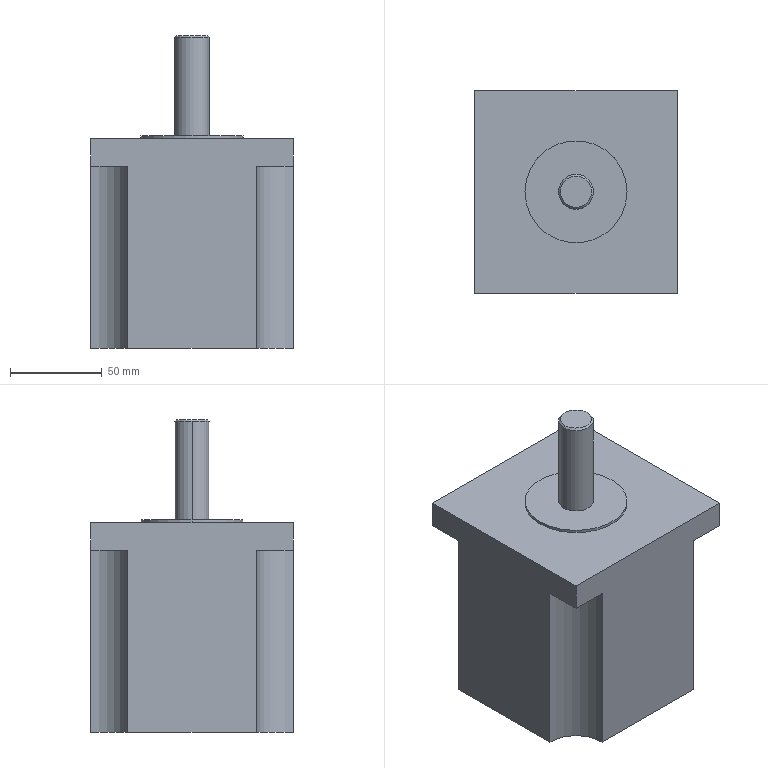Part | STEP file | Guide wheel mechanism revised.sldasm-Part-355 | 1 solid | 22 faces | box 110 x 110 x 170 mm | volume 1274045 mm3 | plane 12 | cylinder 8 | cone 2 | commonest cylinder face diameters 40 x4 19 x2 55.5 x2
STEP:
#1=CARTESIAN_POINT('',(8.5,0.,56.));
#2=VERTEX_POINT('',#1);
#3=CARTESIAN_POINT('',(-8.5,0.,56.));
#4=VERTEX_POINT('',#3);
#5=CARTESIAN_POINT('',(0.,0.,56.));
#6=DIRECTION('',(0.,0.,1.));
#7=DIRECTION('',(1.,0.,0.));
#8=AXIS2_PLACEMENT_3D('',#5,#6,#7);
#9=CIRCLE('',#8,8.5);
#10=EDGE_CURVE('',#2,#4,#9,.T.);
#11=ORIENTED_EDGE('',*,*,#10,.F.);
#12=CARTESIAN_POINT('',(9.5,0.,55.));
#13=VERTEX_POINT('',#12);
#14=CARTESIAN_POINT('',(8.5,0.,56.));
#15=DIRECTION('',(0.7071,0.,-0.7071));
#16=VECTOR('',#15,1000.);
#17=LINE('',#14,#16);
#18=EDGE_CURVE('',#2,#13,#17,.T.);
#19=ORIENTED_EDGE('',*,*,#18,.T.);
#20=CARTESIAN_POINT('',(-9.5,0.,55.));
#21=VERTEX_POINT('',#20);
#22=CARTESIAN_POINT('',(0.,0.,55.));
#23=DIRECTION('',(0.,0.,-1.));
#24=DIRECTION('',(1.,0.,0.));
#25=AXIS2_PLACEMENT_3D('',#22,#23,#24);
#26=CIRCLE('',#25,9.5);
#27=EDGE_CURVE('',#21,#13,#26,.T.);
#28=ORIENTED_EDGE('',*,*,#27,.F.);
#29=CARTESIAN_POINT('',(-8.5,0.,56.));
#30=DIRECTION('',(-0.7071,0.,-0.7071));
#31=VECTOR('',#30,1000.);
#32=LINE('',#29,#31);
#33=EDGE_CURVE('',#4,#21,#32,.T.);
#34=ORIENTED_EDGE('',*,*,#33,.F.);
#35=EDGE_LOOP('',(#11,#19,#28,#34));
#36=FACE_OUTER_BOUND('',#35,.T.);
#37=CARTESIAN_POINT('',(0.,0.,56.));
#38=DIRECTION('',(0.,0.,-1.));
#39=DIRECTION('',(-1.,0.,0.));
#40=AXIS2_PLACEMENT_3D('',#37,#38,#39);
#41=CONICAL_SURFACE('',#40,8.5,0.7854);
#42=ADVANCED_FACE('',(#36),#41,.T.);
#43=ORIENTED_EDGE('',*,*,#27,.T.);
#44=CARTESIAN_POINT('',(9.5,0.,1.5));
#45=VERTEX_POINT('',#44);
#46=CARTESIAN_POINT('',(9.5,0.,56.));
#47=DIRECTION('',(0.,0.,-1.));
#48=VECTOR('',#47,1000.);
#49=LINE('',#46,#48);
#50=EDGE_CURVE('',#13,#45,#49,.T.);
#51=ORIENTED_EDGE('',*,*,#50,.T.);
#52=CARTESIAN_POINT('',(-9.5,0.,1.5));
#53=VERTEX_POINT('',#52);
#54=CARTESIAN_POINT('',(0.,0.,1.5));
#55=DIRECTION('',(0.,0.,1.));
#56=DIRECTION('',(1.,0.,0.));
#57=AXIS2_PLACEMENT_3D('',#54,#55,#56);
#58=CIRCLE('',#57,9.5);
#59=EDGE_CURVE('',#45,#53,#58,.T.);
#60=ORIENTED_EDGE('',*,*,#59,.T.);
#61=CARTESIAN_POINT('',(-9.5,0.,56.));
#62=DIRECTION('',(0.,0.,-1.));
#63=VECTOR('',#62,1000.);
#64=LINE('',#61,#63);
#65=EDGE_CURVE('',#21,#53,#64,.T.);
#66=ORIENTED_EDGE('',*,*,#65,.F.);
#67=EDGE_LOOP('',(#43,#51,#60,#66));
#68=FACE_OUTER_BOUND('',#67,.T.);
#69=CARTESIAN_POINT('',(0.,0.,56.));
#70=DIRECTION('',(0.,0.,-1.));
#71=DIRECTION('',(-1.,0.,0.));
#72=AXIS2_PLACEMENT_3D('',#69,#70,#71);
#73=CYLINDRICAL_SURFACE('',#72,9.5);
#74=ADVANCED_FACE('',(#68),#73,.T.);
#75=CARTESIAN_POINT('',(27.75,0.,1.5));
#76=VERTEX_POINT('',#75);
#77=CARTESIAN_POINT('',(-27.75,0.,1.5));
#78=VERTEX_POINT('',#77);
#79=CARTESIAN_POINT('',(0.,0.,1.5));
#80=DIRECTION('',(0.,0.,1.));
#81=DIRECTION('',(1.,0.,0.));
#82=AXIS2_PLACEMENT_3D('',#79,#80,#81);
#83=CIRCLE('',#82,27.75);
#84=EDGE_CURVE('',#76,#78,#83,.T.);
#85=ORIENTED_EDGE('',*,*,#84,.F.);
#86=CARTESIAN_POINT('',(27.75,0.,0.));
#87=VERTEX_POINT('',#86);
#88=CARTESIAN_POINT('',(27.75,0.,1.5));
#89=DIRECTION('',(0.,0.,-1.));
#90=VECTOR('',#89,1000.);
#91=LINE('',#88,#90);
#92=EDGE_CURVE('',#76,#87,#91,.T.);
#93=ORIENTED_EDGE('',*,*,#92,.T.);
#94=CARTESIAN_POINT('',(-27.75,0.,0.));
#95=VERTEX_POINT('',#94);
#96=CARTESIAN_POINT('',(0.,0.,0.));
#97=DIRECTION('',(0.,0.,1.));
#98=DIRECTION('',(1.,0.,0.));
#99=AXIS2_PLACEMENT_3D('',#96,#97,#98);
#100=CIRCLE('',#99,27.75);
#101=EDGE_CURVE('',#87,#95,#100,.T.);
#102=ORIENTED_EDGE('',*,*,#101,.T.);
#103=CARTESIAN_POINT('',(-27.75,0.,1.5));
#104=DIRECTION('',(0.,0.,-1.));
#105=VECTOR('',#104,1000.);
#106=LINE('',#103,#105);
#107=EDGE_CURVE('',#78,#95,#106,.T.);
#108=ORIENTED_EDGE('',*,*,#107,.F.);
#109=EDGE_LOOP('',(#85,#93,#102,#108));
#110=FACE_OUTER_BOUND('',#109,.T.);
#111=CARTESIAN_POINT('',(0.,0.,1.5));
#112=DIRECTION('',(0.,0.,-1.));
#113=DIRECTION('',(-1.,0.,0.));
#114=AXIS2_PLACEMENT_3D('',#111,#112,#113);
#115=CYLINDRICAL_SURFACE('',#114,27.75);
#116=ADVANCED_FACE('',(#110),#115,.T.);
#117=CARTESIAN_POINT('',(-55.,-55.,0.));
#118=VERTEX_POINT('',#117);
#119=CARTESIAN_POINT('',(-55.,55.,0.));
#120=VERTEX_POINT('',#119);
#121=CARTESIAN_POINT('',(-55.,0.,0.));
#122=DIRECTION('',(0.,1.,0.));
#123=VECTOR('',#122,1000.);
#124=LINE('',#121,#123);
#125=EDGE_CURVE('',#118,#120,#124,.T.);
#126=ORIENTED_EDGE('',*,*,#125,.F.);
#127=CARTESIAN_POINT('',(55.,-55.,0.));
#128=VERTEX_POINT('',#127);
#129=CARTESIAN_POINT('',(0.,-55.,0.));
#130=DIRECTION('',(-1.,0.,0.));
#131=VECTOR('',#130,1000.);
#132=LINE('',#129,#131);
#133=EDGE_CURVE('',#128,#118,#132,.T.);
#134=ORIENTED_EDGE('',*,*,#133,.F.);
#135=CARTESIAN_POINT('',(55.,55.,0.));
#136=VERTEX_POINT('',#135);
#137=CARTESIAN_POINT('',(55.,0.,0.));
#138=DIRECTION('',(0.,1.,0.));
#139=VECTOR('',#138,1000.);
#140=LINE('',#137,#139);
#141=EDGE_CURVE('',#128,#136,#140,.T.);
#142=ORIENTED_EDGE('',*,*,#141,.T.);
#143=CARTESIAN_POINT('',(0.,55.,0.));
#144=DIRECTION('',(-1.,0.,0.));
#145=VECTOR('',#144,1000.);
#146=LINE('',#143,#145);
#147=EDGE_CURVE('',#136,#120,#146,.T.);
#148=ORIENTED_EDGE('',*,*,#147,.T.);
#149=EDGE_LOOP('',(#126,#134,#142,#148));
#150=FACE_OUTER_BOUND('',#149,.T.);
#151=CARTESIAN_POINT('',(0.,0.,0.));
#152=DIRECTION('',(0.,0.,1.));
#153=DIRECTION('',(1.,0.,0.));
#154=AXIS2_PLACEMENT_3D('',#151,#152,#153);
#155=CIRCLE('',#154,27.75);
#156=EDGE_CURVE('',#95,#87,#155,.T.);
#157=ORIENTED_EDGE('',*,*,#156,.F.);
#158=ORIENTED_EDGE('',*,*,#101,.F.);
#159=EDGE_LOOP('',(#157,#158));
#160=FACE_BOUND('',#159,.T.);
#161=CARTESIAN_POINT('',(0.,0.,0.));
#162=DIRECTION('',(0.,0.,1.));
#163=DIRECTION('',(1.,0.,0.));
#164=AXIS2_PLACEMENT_3D('',#161,#162,#163);
#165=PLANE('',#164);
#166=ADVANCED_FACE('',(#150,#160),#165,.T.);
#167=CARTESIAN_POINT('',(-55.,-35.,-15.));
#168=VERTEX_POINT('',#167);
#169=CARTESIAN_POINT('',(-35.,-55.,-15.));
#170=VERTEX_POINT('',#169);
#171=CARTESIAN_POINT('',(-55.,-55.,-15.));
#172=DIRECTION('',(0.,0.,-1.));
#173=DIRECTION('',(1.,0.,0.));
#174=AXIS2_PLACEMENT_3D('',#171,#172,#173);
#175=CIRCLE('',#174,20.);
#176=EDGE_CURVE('',#168,#170,#175,.T.);
#177=ORIENTED_EDGE('',*,*,#176,.F.);
#178=CARTESIAN_POINT('',(-55.,-35.,-114.));
#179=VERTEX_POINT('',#178);
#180=CARTESIAN_POINT('',(-55.,-35.,-114.));
#181=DIRECTION('',(0.,0.,1.));
#182=VECTOR('',#181,1000.);
#183=LINE('',#180,#182);
#184=EDGE_CURVE('',#179,#168,#183,.T.);
#185=ORIENTED_EDGE('',*,*,#184,.F.);
#186=CARTESIAN_POINT('',(-35.,-55.,-114.));
#187=VERTEX_POINT('',#186);
#188=CARTESIAN_POINT('',(-55.,-55.,-114.));
#189=DIRECTION('',(0.,0.,1.));
#190=DIRECTION('',(1.,0.,0.));
#191=AXIS2_PLACEMENT_3D('',#188,#189,#190);
#192=CIRCLE('',#191,20.);
#193=EDGE_CURVE('',#187,#179,#192,.T.);
#194=ORIENTED_EDGE('',*,*,#193,.F.);
#195=CARTESIAN_POINT('',(-35.,-55.,-114.));
#196=DIRECTION('',(0.,0.,1.));
#197=VECTOR('',#196,1000.);
#198=LINE('',#195,#197);
#199=EDGE_CURVE('',#187,#170,#198,.T.);
#200=ORIENTED_EDGE('',*,*,#199,.T.);
#201=EDGE_LOOP('',(#177,#185,#194,#200));
#202=FACE_OUTER_BOUND('',#201,.T.);
#203=CARTESIAN_POINT('',(-55.,-55.,-114.));
#204=DIRECTION('',(0.,0.,1.));
#205=DIRECTION('',(1.,0.,0.));
#206=AXIS2_PLACEMENT_3D('',#203,#204,#205);
#207=CYLINDRICAL_SURFACE('',#206,20.);
#208=ADVANCED_FACE('',(#202),#207,.F.);
#209=CARTESIAN_POINT('',(-35.,55.,-15.));
#210=VERTEX_POINT('',#209);
#211=CARTESIAN_POINT('',(-55.,35.,-15.));
#212=VERTEX_POINT('',#211);
#213=CARTESIAN_POINT('',(-55.,55.,-15.));
#214=DIRECTION('',(0.,0.,-1.));
#215=DIRECTION('',(1.,0.,0.));
#216=AXIS2_PLACEMENT_3D('',#213,#214,#215);
#217=CIRCLE('',#216,20.);
#218=EDGE_CURVE('',#210,#212,#217,.T.);
#219=ORIENTED_EDGE('',*,*,#218,.F.);
#220=CARTESIAN_POINT('',(-35.,55.,-114.));
#221=VERTEX_POINT('',#220);
#222=CARTESIAN_POINT('',(-35.,55.,-114.));
#223=DIRECTION('',(0.,0.,1.));
#224=VECTOR('',#223,1000.);
#225=LINE('',#222,#224);
#226=EDGE_CURVE('',#221,#210,#225,.T.);
#227=ORIENTED_EDGE('',*,*,#226,.F.);
#228=CARTESIAN_POINT('',(-55.,35.,-114.));
#229=VERTEX_POINT('',#228);
#230=CARTESIAN_POINT('',(-55.,55.,-114.));
#231=DIRECTION('',(0.,0.,1.));
#232=DIRECTION('',(1.,0.,0.));
#233=AXIS2_PLACEMENT_3D('',#230,#231,#232);
#234=CIRCLE('',#233,20.);
#235=EDGE_CURVE('',#229,#221,#234,.T.);
#236=ORIENTED_EDGE('',*,*,#235,.F.);
#237=CARTESIAN_POINT('',(-55.,35.,-114.));
#238=DIRECTION('',(0.,0.,1.));
#239=VECTOR('',#238,1000.);
#240=LINE('',#237,#239);
#241=EDGE_CURVE('',#229,#212,#240,.T.);
#242=ORIENTED_EDGE('',*,*,#241,.T.);
#243=EDGE_LOOP('',(#219,#227,#236,#242));
#244=FACE_OUTER_BOUND('',#243,.T.);
#245=CARTESIAN_POINT('',(-55.,55.,-114.));
#246=DIRECTION('',(0.,0.,1.));
#247=DIRECTION('',(1.,0.,0.));
#248=AXIS2_PLACEMENT_3D('',#245,#246,#247);
#249=CYLINDRICAL_SURFACE('',#248,20.);
#250=ADVANCED_FACE('',(#244),#249,.F.);
#251=CARTESIAN_POINT('',(55.,35.,-15.));
#252=VERTEX_POINT('',#251);
#253=CARTESIAN_POINT('',(35.,55.,-15.));
#254=VERTEX_POINT('',#253);
#255=CARTESIAN_POINT('',(55.,55.,-15.));
#256=DIRECTION('',(0.,0.,-1.));
#257=DIRECTION('',(1.,0.,0.));
#258=AXIS2_PLACEMENT_3D('',#255,#256,#257);
#259=CIRCLE('',#258,20.);
#260=EDGE_CURVE('',#252,#254,#259,.T.);
#261=ORIENTED_EDGE('',*,*,#260,.F.);
#262=CARTESIAN_POINT('',(55.,35.,-114.));
#263=VERTEX_POINT('',#262);
#264=CARTESIAN_POINT('',(55.,35.,-114.));
#265=DIRECTION('',(0.,0.,1.));
#266=VECTOR('',#265,1000.);
#267=LINE('',#264,#266);
#268=EDGE_CURVE('',#263,#252,#267,.T.);
#269=ORIENTED_EDGE('',*,*,#268,.F.);
#270=CARTESIAN_POINT('',(35.,55.,-114.));
#271=VERTEX_POINT('',#270);
#272=CARTESIAN_POINT('',(55.,55.,-114.));
#273=DIRECTION('',(0.,0.,1.));
#274=DIRECTION('',(1.,0.,0.));
#275=AXIS2_PLACEMENT_3D('',#272,#273,#274);
#276=CIRCLE('',#275,20.);
#277=EDGE_CURVE('',#271,#263,#276,.T.);
#278=ORIENTED_EDGE('',*,*,#277,.F.);
#279=CARTESIAN_POINT('',(35.,55.,-114.));
#280=DIRECTION('',(0.,0.,1.));
#281=VECTOR('',#280,1000.);
#282=LINE('',#279,#281);
#283=EDGE_CURVE('',#271,#254,#282,.T.);
#284=ORIENTED_EDGE('',*,*,#283,.T.);
#285=EDGE_LOOP('',(#261,#269,#278,#284));
#286=FACE_OUTER_BOUND('',#285,.T.);
#287=CARTESIAN_POINT('',(55.,55.,-114.));
#288=DIRECTION('',(0.,0.,1.));
#289=DIRECTION('',(1.,0.,0.));
#290=AXIS2_PLACEMENT_3D('',#287,#288,#289);
#291=CYLINDRICAL_SURFACE('',#290,20.);
#292=ADVANCED_FACE('',(#286),#291,.F.);
#293=CARTESIAN_POINT('',(35.,-55.,-15.));
#294=VERTEX_POINT('',#293);
#295=CARTESIAN_POINT('',(55.,-35.,-15.));
#296=VERTEX_POINT('',#295);
#297=CARTESIAN_POINT('',(55.,-55.,-15.));
#298=DIRECTION('',(0.,0.,-1.));
#299=DIRECTION('',(1.,0.,0.));
#300=AXIS2_PLACEMENT_3D('',#297,#298,#299);
#301=CIRCLE('',#300,20.);
#302=EDGE_CURVE('',#294,#296,#301,.T.);
#303=ORIENTED_EDGE('',*,*,#302,.F.);
#304=CARTESIAN_POINT('',(35.,-55.,-114.));
#305=VERTEX_POINT('',#304);
#306=CARTESIAN_POINT('',(35.,-55.,-114.));
#307=DIRECTION('',(0.,0.,1.));
#308=VECTOR('',#307,1000.);
#309=LINE('',#306,#308);
#310=EDGE_CURVE('',#305,#294,#309,.T.);
#311=ORIENTED_EDGE('',*,*,#310,.F.);
#312=CARTESIAN_POINT('',(55.,-35.,-114.));
#313=VERTEX_POINT('',#312);
#314=CARTESIAN_POINT('',(55.,-55.,-114.));
#315=DIRECTION('',(0.,0.,1.));
#316=DIRECTION('',(1.,0.,0.));
#317=AXIS2_PLACEMENT_3D('',#314,#315,#316);
#318=CIRCLE('',#317,20.);
#319=EDGE_CURVE('',#313,#305,#318,.T.);
#320=ORIENTED_EDGE('',*,*,#319,.F.);
#321=CARTESIAN_POINT('',(55.,-35.,-114.));
#322=DIRECTION('',(0.,0.,1.));
#323=VECTOR('',#322,1000.);
#324=LINE('',#321,#323);
#325=EDGE_CURVE('',#313,#296,#324,.T.);
#326=ORIENTED_EDGE('',*,*,#325,.T.);
#327=EDGE_LOOP('',(#303,#311,#320,#326));
#328=FACE_OUTER_BOUND('',#327,.T.);
#329=CARTESIAN_POINT('',(55.,-55.,-114.));
#330=DIRECTION('',(0.,0.,1.));
#331=DIRECTION('',(1.,0.,0.));
#332=AXIS2_PLACEMENT_3D('',#329,#330,#331);
#333=CYLINDRICAL_SURFACE('',#332,20.);
#334=ADVANCED_FACE('',(#328),#333,.F.);
#335=ORIENTED_EDGE('',*,*,#125,.T.);
#336=CARTESIAN_POINT('',(-55.,55.,-15.));
#337=VERTEX_POINT('',#336);
#338=CARTESIAN_POINT('',(-55.,55.,-15.));
#339=DIRECTION('',(0.,0.,1.));
#340=VECTOR('',#339,1000.);
#341=LINE('',#338,#340);
#342=EDGE_CURVE('',#337,#120,#341,.T.);
#343=ORIENTED_EDGE('',*,*,#342,.F.);
#344=CARTESIAN_POINT('',(-55.,0.,-15.));
#345=DIRECTION('',(0.,1.,0.));
#346=VECTOR('',#345,1000.);
#347=LINE('',#344,#346);
#348=EDGE_CURVE('',#212,#337,#347,.T.);
#349=ORIENTED_EDGE('',*,*,#348,.F.);
#350=ORIENTED_EDGE('',*,*,#241,.F.);
#351=CARTESIAN_POINT('',(-55.,0.,-114.));
#352=DIRECTION('',(0.,1.,0.));
#353=VECTOR('',#352,1000.);
#354=LINE('',#351,#353);
#355=EDGE_CURVE('',#179,#229,#354,.T.);
#356=ORIENTED_EDGE('',*,*,#355,.F.);
#357=ORIENTED_EDGE('',*,*,#184,.T.);
#358=CARTESIAN_POINT('',(-55.,-55.,-15.));
#359=VERTEX_POINT('',#358);
#360=CARTESIAN_POINT('',(-55.,0.,-15.));
#361=DIRECTION('',(0.,1.,0.));
#362=VECTOR('',#361,1000.);
#363=LINE('',#360,#362);
#364=EDGE_CURVE('',#359,#168,#363,.T.);
#365=ORIENTED_EDGE('',*,*,#364,.F.);
#366=CARTESIAN_POINT('',(-55.,-55.,-15.));
#367=DIRECTION('',(0.,0.,1.));
#368=VECTOR('',#367,1000.);
#369=LINE('',#366,#368);
#370=EDGE_CURVE('',#359,#118,#369,.T.);
#371=ORIENTED_EDGE('',*,*,#370,.T.);
#372=EDGE_LOOP('',(#335,#343,#349,#350,#356,#357,#365,#371));
#373=FACE_OUTER_BOUND('',#372,.T.);
#374=CARTESIAN_POINT('',(-55.,0.,-114.));
#375=DIRECTION('',(1.,0.,0.));
#376=DIRECTION('',(0.,0.,-1.));
#377=AXIS2_PLACEMENT_3D('',#374,#375,#376);
#378=PLANE('',#377);
#379=ADVANCED_FACE('',(#373),#378,.F.);
#380=CARTESIAN_POINT('',(55.,55.,-15.));
#381=VERTEX_POINT('',#380);
#382=CARTESIAN_POINT('',(0.,55.,-15.));
#383=DIRECTION('',(-1.,0.,0.));
#384=VECTOR('',#383,1000.);
#385=LINE('',#382,#384);
#386=EDGE_CURVE('',#381,#254,#385,.T.);
#387=ORIENTED_EDGE('',*,*,#386,.T.);
#388=ORIENTED_EDGE('',*,*,#283,.F.);
#389=CARTESIAN_POINT('',(0.,55.,-114.));
#390=DIRECTION('',(-1.,0.,0.));
#391=VECTOR('',#390,1000.);
#392=LINE('',#389,#391);
#393=EDGE_CURVE('',#271,#221,#392,.T.);
#394=ORIENTED_EDGE('',*,*,#393,.T.);
#395=ORIENTED_EDGE('',*,*,#226,.T.);
#396=CARTESIAN_POINT('',(0.,55.,-15.));
#397=DIRECTION('',(-1.,0.,0.));
#398=VECTOR('',#397,1000.);
#399=LINE('',#396,#398);
#400=EDGE_CURVE('',#210,#337,#399,.T.);
#401=ORIENTED_EDGE('',*,*,#400,.T.);
#402=ORIENTED_EDGE('',*,*,#342,.T.);
#403=ORIENTED_EDGE('',*,*,#147,.F.);
#404=CARTESIAN_POINT('',(55.,55.,-15.));
#405=DIRECTION('',(0.,0.,1.));
#406=VECTOR('',#405,1000.);
#407=LINE('',#404,#406);
#408=EDGE_CURVE('',#381,#136,#407,.T.);
#409=ORIENTED_EDGE('',*,*,#408,.F.);
#410=EDGE_LOOP('',(#387,#388,#394,#395,#401,#402,#403,#409));
#411=FACE_OUTER_BOUND('',#410,.T.);
#412=CARTESIAN_POINT('',(0.,55.,-114.));
#413=DIRECTION('',(0.,1.,0.));
#414=DIRECTION('',(-1.,0.,0.));
#415=AXIS2_PLACEMENT_3D('',#412,#413,#414);
#416=PLANE('',#415);
#417=ADVANCED_FACE('',(#411),#416,.T.);
#418=CARTESIAN_POINT('',(55.,-55.,-15.));
#419=VERTEX_POINT('',#418);
#420=CARTESIAN_POINT('',(55.,0.,-15.));
#421=DIRECTION('',(0.,1.,0.));
#422=VECTOR('',#421,1000.);
#423=LINE('',#420,#422);
#424=EDGE_CURVE('',#419,#296,#423,.T.);
#425=ORIENTED_EDGE('',*,*,#424,.T.);
#426=ORIENTED_EDGE('',*,*,#325,.F.);
#427=CARTESIAN_POINT('',(55.,0.,-114.));
#428=DIRECTION('',(0.,1.,0.));
#429=VECTOR('',#428,1000.);
#430=LINE('',#427,#429);
#431=EDGE_CURVE('',#313,#263,#430,.T.);
#432=ORIENTED_EDGE('',*,*,#431,.T.);
#433=ORIENTED_EDGE('',*,*,#268,.T.);
#434=CARTESIAN_POINT('',(55.,0.,-15.));
#435=DIRECTION('',(0.,1.,0.));
#436=VECTOR('',#435,1000.);
#437=LINE('',#434,#436);
#438=EDGE_CURVE('',#252,#381,#437,.T.);
#439=ORIENTED_EDGE('',*,*,#438,.T.);
#440=ORIENTED_EDGE('',*,*,#408,.T.);
#441=ORIENTED_EDGE('',*,*,#141,.F.);
#442=CARTESIAN_POINT('',(55.,-55.,-15.));
#443=DIRECTION('',(0.,0.,1.));
#444=VECTOR('',#443,1000.);
#445=LINE('',#442,#444);
#446=EDGE_CURVE('',#419,#128,#445,.T.);
#447=ORIENTED_EDGE('',*,*,#446,.F.);
#448=EDGE_LOOP('',(#425,#426,#432,#433,#439,#440,#441,#447));
#449=FACE_OUTER_BOUND('',#448,.T.);
#450=CARTESIAN_POINT('',(55.,0.,-114.));
#451=DIRECTION('',(1.,0.,0.));
#452=DIRECTION('',(0.,0.,-1.));
#453=AXIS2_PLACEMENT_3D('',#450,#451,#452);
#454=PLANE('',#453);
#455=ADVANCED_FACE('',(#449),#454,.T.);
#456=ORIENTED_EDGE('',*,*,#133,.T.);
#457=ORIENTED_EDGE('',*,*,#370,.F.);
#458=CARTESIAN_POINT('',(0.,-55.,-15.));
#459=DIRECTION('',(-1.,0.,0.));
#460=VECTOR('',#459,1000.);
#461=LINE('',#458,#460);
#462=EDGE_CURVE('',#170,#359,#461,.T.);
#463=ORIENTED_EDGE('',*,*,#462,.F.);
#464=ORIENTED_EDGE('',*,*,#199,.F.);
#465=CARTESIAN_POINT('',(0.,-55.,-114.));
#466=DIRECTION('',(-1.,0.,0.));
#467=VECTOR('',#466,1000.);
#468=LINE('',#465,#467);
#469=EDGE_CURVE('',#305,#187,#468,.T.);
#470=ORIENTED_EDGE('',*,*,#469,.F.);
#471=ORIENTED_EDGE('',*,*,#310,.T.);
#472=CARTESIAN_POINT('',(0.,-55.,-15.));
#473=DIRECTION('',(-1.,0.,0.));
#474=VECTOR('',#473,1000.);
#475=LINE('',#472,#474);
#476=EDGE_CURVE('',#419,#294,#475,.T.);
#477=ORIENTED_EDGE('',*,*,#476,.F.);
#478=ORIENTED_EDGE('',*,*,#446,.T.);
#479=EDGE_LOOP('',(#456,#457,#463,#464,#470,#471,#477,#478));
#480=FACE_OUTER_BOUND('',#479,.T.);
#481=CARTESIAN_POINT('',(0.,-55.,-114.));
#482=DIRECTION('',(0.,1.,0.));
#483=DIRECTION('',(-1.,0.,0.));
#484=AXIS2_PLACEMENT_3D('',#481,#482,#483);
#485=PLANE('',#484);
#486=ADVANCED_FACE('',(#480),#485,.F.);
#487=ORIENTED_EDGE('',*,*,#193,.T.);
#488=ORIENTED_EDGE('',*,*,#355,.T.);
#489=ORIENTED_EDGE('',*,*,#235,.T.);
#490=ORIENTED_EDGE('',*,*,#393,.F.);
#491=ORIENTED_EDGE('',*,*,#277,.T.);
#492=ORIENTED_EDGE('',*,*,#431,.F.);
#493=ORIENTED_EDGE('',*,*,#319,.T.);
#494=ORIENTED_EDGE('',*,*,#469,.T.);
#495=EDGE_LOOP('',(#487,#488,#489,#490,#491,#492,#493,#494));
#496=FACE_OUTER_BOUND('',#495,.T.);
#497=CARTESIAN_POINT('',(0.,0.,-114.));
#498=DIRECTION('',(0.,0.,1.));
#499=DIRECTION('',(1.,0.,0.));
#500=AXIS2_PLACEMENT_3D('',#497,#498,#499);
#501=PLANE('',#500);
#502=ADVANCED_FACE('',(#496),#501,.F.);
#503=ORIENTED_EDGE('',*,*,#476,.T.);
#504=ORIENTED_EDGE('',*,*,#302,.T.);
#505=ORIENTED_EDGE('',*,*,#424,.F.);
#506=EDGE_LOOP('',(#503,#504,#505));
#507=FACE_OUTER_BOUND('',#506,.T.);
#508=CARTESIAN_POINT('',(0.,0.,-15.));
#509=DIRECTION('',(0.,0.,1.));
#510=DIRECTION('',(1.,0.,0.));
#511=AXIS2_PLACEMENT_3D('',#508,#509,#510);
#512=PLANE('',#511);
#513=ADVANCED_FACE('',(#507),#512,.F.);
#514=ORIENTED_EDGE('',*,*,#438,.F.);
#515=ORIENTED_EDGE('',*,*,#260,.T.);
#516=ORIENTED_EDGE('',*,*,#386,.F.);
#517=EDGE_LOOP('',(#514,#515,#516));
#518=FACE_OUTER_BOUND('',#517,.T.);
#519=CARTESIAN_POINT('',(0.,0.,-15.));
#520=DIRECTION('',(0.,0.,1.));
#521=DIRECTION('',(1.,0.,0.));
#522=AXIS2_PLACEMENT_3D('',#519,#520,#521);
#523=PLANE('',#522);
#524=ADVANCED_FACE('',(#518),#523,.F.);
#525=ORIENTED_EDGE('',*,*,#400,.F.);
#526=ORIENTED_EDGE('',*,*,#218,.T.);
#527=ORIENTED_EDGE('',*,*,#348,.T.);
#528=EDGE_LOOP('',(#525,#526,#527));
#529=FACE_OUTER_BOUND('',#528,.T.);
#530=CARTESIAN_POINT('',(0.,0.,-15.));
#531=DIRECTION('',(0.,0.,1.));
#532=DIRECTION('',(1.,0.,0.));
#533=AXIS2_PLACEMENT_3D('',#530,#531,#532);
#534=PLANE('',#533);
#535=ADVANCED_FACE('',(#529),#534,.F.);
#536=ORIENTED_EDGE('',*,*,#364,.T.);
#537=ORIENTED_EDGE('',*,*,#176,.T.);
#538=ORIENTED_EDGE('',*,*,#462,.T.);
#539=EDGE_LOOP('',(#536,#537,#538));
#540=FACE_OUTER_BOUND('',#539,.T.);
#541=CARTESIAN_POINT('',(0.,0.,-15.));
#542=DIRECTION('',(0.,0.,1.));
#543=DIRECTION('',(1.,0.,0.));
#544=AXIS2_PLACEMENT_3D('',#541,#542,#543);
#545=PLANE('',#544);
#546=ADVANCED_FACE('',(#540),#545,.F.);
#547=CARTESIAN_POINT('',(0.,0.,1.5));
#548=DIRECTION('',(0.,0.,1.));
#549=DIRECTION('',(1.,0.,0.));
#550=AXIS2_PLACEMENT_3D('',#547,#548,#549);
#551=CIRCLE('',#550,27.75);
#552=EDGE_CURVE('',#78,#76,#551,.T.);
#553=ORIENTED_EDGE('',*,*,#552,.T.);
#554=ORIENTED_EDGE('',*,*,#84,.T.);
#555=EDGE_LOOP('',(#553,#554));
#556=FACE_OUTER_BOUND('',#555,.T.);
#557=CARTESIAN_POINT('',(0.,0.,1.5));
#558=DIRECTION('',(0.,0.,1.));
#559=DIRECTION('',(1.,0.,0.));
#560=AXIS2_PLACEMENT_3D('',#557,#558,#559);
#561=CIRCLE('',#560,9.5);
#562=EDGE_CURVE('',#53,#45,#561,.T.);
#563=ORIENTED_EDGE('',*,*,#562,.F.);
#564=ORIENTED_EDGE('',*,*,#59,.F.);
#565=EDGE_LOOP('',(#563,#564));
#566=FACE_BOUND('',#565,.T.);
#567=CARTESIAN_POINT('',(0.,0.,1.5));
#568=DIRECTION('',(0.,0.,1.));
#569=DIRECTION('',(1.,0.,0.));
#570=AXIS2_PLACEMENT_3D('',#567,#568,#569);
#571=PLANE('',#570);
#572=ADVANCED_FACE('',(#556,#566),#571,.T.);
#573=ORIENTED_EDGE('',*,*,#92,.F.);
#574=ORIENTED_EDGE('',*,*,#552,.F.);
#575=ORIENTED_EDGE('',*,*,#107,.T.);
#576=ORIENTED_EDGE('',*,*,#156,.T.);
#577=EDGE_LOOP('',(#573,#574,#575,#576));
#578=FACE_OUTER_BOUND('',#577,.T.);
#579=CARTESIAN_POINT('',(0.,0.,1.5));
#580=DIRECTION('',(0.,0.,-1.));
#581=DIRECTION('',(-1.,0.,0.));
#582=AXIS2_PLACEMENT_3D('',#579,#580,#581);
#583=CYLINDRICAL_SURFACE('',#582,27.75);
#584=ADVANCED_FACE('',(#578),#583,.T.);
#585=CARTESIAN_POINT('',(0.,0.,56.));
#586=DIRECTION('',(0.,0.,1.));
#587=DIRECTION('',(1.,0.,0.));
#588=AXIS2_PLACEMENT_3D('',#585,#586,#587);
#589=CIRCLE('',#588,8.5);
#590=EDGE_CURVE('',#4,#2,#589,.T.);
#591=ORIENTED_EDGE('',*,*,#590,.T.);
#592=ORIENTED_EDGE('',*,*,#10,.T.);
#593=EDGE_LOOP('',(#591,#592));
#594=FACE_OUTER_BOUND('',#593,.T.);
#595=CARTESIAN_POINT('',(0.,0.,56.));
#596=DIRECTION('',(0.,0.,1.));
#597=DIRECTION('',(1.,0.,0.));
#598=AXIS2_PLACEMENT_3D('',#595,#596,#597);
#599=PLANE('',#598);
#600=ADVANCED_FACE('',(#594),#599,.T.);
#601=ORIENTED_EDGE('',*,*,#50,.F.);
#602=CARTESIAN_POINT('',(0.,0.,55.));
#603=DIRECTION('',(0.,0.,-1.));
#604=DIRECTION('',(1.,0.,0.));
#605=AXIS2_PLACEMENT_3D('',#602,#603,#604);
#606=CIRCLE('',#605,9.5);
#607=EDGE_CURVE('',#13,#21,#606,.T.);
#608=ORIENTED_EDGE('',*,*,#607,.T.);
#609=ORIENTED_EDGE('',*,*,#65,.T.);
#610=ORIENTED_EDGE('',*,*,#562,.T.);
#611=EDGE_LOOP('',(#601,#608,#609,#610));
#612=FACE_OUTER_BOUND('',#611,.T.);
#613=CARTESIAN_POINT('',(0.,0.,56.));
#614=DIRECTION('',(0.,0.,-1.));
#615=DIRECTION('',(-1.,0.,0.));
#616=AXIS2_PLACEMENT_3D('',#613,#614,#615);
#617=CYLINDRICAL_SURFACE('',#616,9.5);
#618=ADVANCED_FACE('',(#612),#617,.T.);
#619=ORIENTED_EDGE('',*,*,#18,.F.);
#620=ORIENTED_EDGE('',*,*,#590,.F.);
#621=ORIENTED_EDGE('',*,*,#33,.T.);
#622=ORIENTED_EDGE('',*,*,#607,.F.);
#623=EDGE_LOOP('',(#619,#620,#621,#622));
#624=FACE_OUTER_BOUND('',#623,.T.);
#625=CARTESIAN_POINT('',(0.,0.,56.));
#626=DIRECTION('',(0.,0.,-1.));
#627=DIRECTION('',(-1.,0.,0.));
#628=AXIS2_PLACEMENT_3D('',#625,#626,#627);
#629=CONICAL_SURFACE('',#628,8.5,0.7854);
#630=ADVANCED_FACE('',(#624),#629,.T.);
#631=CLOSED_SHELL('',(#42,#74,#116,#166,#208,#250,#292,#334,#379,#417,#455,#486,#502,#513,#524,#535,#546,#572,#584,#600,#618,#630));
#632=MANIFOLD_SOLID_BREP('',#631);
#633=CARTESIAN_POINT('',(0.,0.,0.));
#634=DIRECTION('',(0.,0.,1.));
#635=DIRECTION('',(1.,0.,0.));
#636=AXIS2_PLACEMENT_3D('',#633,#634,#635);
#637=(LENGTH_UNIT()NAMED_UNIT(*)SI_UNIT(.MILLI.,.METRE.));
#638=UNCERTAINTY_MEASURE_WITH_UNIT(LENGTH_MEASURE(0.00001),#637,'','');
#639=(NAMED_UNIT(*)PLANE_ANGLE_UNIT()SI_UNIT($,.RADIAN.));
#640=(NAMED_UNIT(*)SI_UNIT($,.STERADIAN.)SOLID_ANGLE_UNIT());
#641=(GEOMETRIC_REPRESENTATION_CONTEXT(3)GLOBAL_UNCERTAINTY_ASSIGNED_CONTEXT((#638))GLOBAL_UNIT_ASSIGNED_CONTEXT((#637,#639,#640))REPRESENTATION_CONTEXT('',''));
#642=ADVANCED_BREP_SHAPE_REPRESENTATION('',(#632,#636),#641);